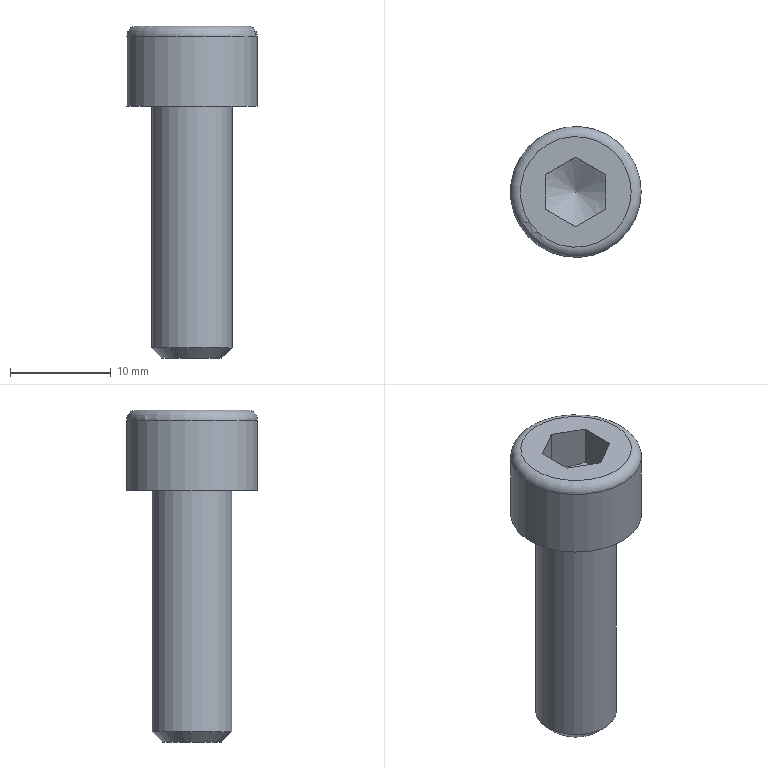Part | NX | features solid 2 | 1 solid | 14 faces | box 13 x 13 x 33 mm | volume 2150 mm3 | plane 9 | cylinder 2 | cone 2 | torus 1 | commonest cylinder face diameters 8 x1 13 x1
STEP:
#1=CARTESIAN_POINT('',(631.,-240.,30.));
#2=VERTEX_POINT('',#1);
#3=CARTESIAN_POINT('',(635.,-240.,30.));
#4=DIRECTION('',(0.,0.,-1.));
#5=DIRECTION('',(-1.,0.,0.));
#6=AXIS2_PLACEMENT_3D('',#3,#4,#5);
#7=CIRCLE('',#6,4.);
#8=EDGE_CURVE('',#2,#2,#7,.T.);
#9=ORIENTED_EDGE('',*,*,#8,.T.);
#10=EDGE_LOOP('',(#9));
#11=FACE_BOUND('',#10,.T.);
#12=CARTESIAN_POINT('',(631.,-240.,6.));
#13=VERTEX_POINT('',#12);
#14=CARTESIAN_POINT('',(635.,-240.,6.));
#15=DIRECTION('',(0.,0.,-1.));
#16=DIRECTION('',(-1.,0.,0.));
#17=AXIS2_PLACEMENT_3D('',#14,#15,#16);
#18=CIRCLE('',#17,4.);
#19=EDGE_CURVE('',#13,#13,#18,.F.);
#20=ORIENTED_EDGE('',*,*,#19,.T.);
#21=EDGE_LOOP('',(#20));
#22=FACE_BOUND('',#21,.T.);
#23=CARTESIAN_POINT('',(635.,-240.,30.));
#24=DIRECTION('',(0.,0.,-1.));
#25=DIRECTION('',(-1.,0.,0.));
#26=AXIS2_PLACEMENT_3D('',#23,#24,#25);
#27=CYLINDRICAL_SURFACE('',#26,4.);
#28=ADVANCED_FACE('',(#11,#22),#27,.T.);
#29=CARTESIAN_POINT('',(640.5,-240.,38.));
#30=VERTEX_POINT('',#29);
#31=CARTESIAN_POINT('',(635.,-240.,38.));
#32=DIRECTION('',(0.,0.,1.));
#33=DIRECTION('',(1.,0.,0.));
#34=AXIS2_PLACEMENT_3D('',#31,#32,#33);
#35=CIRCLE('',#34,5.5);
#36=EDGE_CURVE('',#30,#30,#35,.T.);
#37=ORIENTED_EDGE('',*,*,#36,.T.);
#38=EDGE_LOOP('',(#37));
#39=FACE_BOUND('',#38,.T.);
#40=CARTESIAN_POINT('',(638.,-241.732,38.));
#41=VERTEX_POINT('',#40);
#42=CARTESIAN_POINT('',(635.,-243.464,38.));
#43=VERTEX_POINT('',#42);
#44=CARTESIAN_POINT('',(638.,-241.732,38.));
#45=DIRECTION('',(-0.866,-0.5,0.));
#46=VECTOR('',#45,1000.);
#47=LINE('',#44,#46);
#48=EDGE_CURVE('',#41,#43,#47,.T.);
#49=ORIENTED_EDGE('',*,*,#48,.T.);
#50=CARTESIAN_POINT('',(632.,-241.732,38.));
#51=VERTEX_POINT('',#50);
#52=CARTESIAN_POINT('',(635.,-243.464,38.));
#53=DIRECTION('',(-0.866,0.5,0.));
#54=VECTOR('',#53,1000.);
#55=LINE('',#52,#54);
#56=EDGE_CURVE('',#43,#51,#55,.T.);
#57=ORIENTED_EDGE('',*,*,#56,.T.);
#58=CARTESIAN_POINT('',(632.,-238.268,38.));
#59=VERTEX_POINT('',#58);
#60=CARTESIAN_POINT('',(632.,-241.732,38.));
#61=DIRECTION('',(0.,1.,0.));
#62=VECTOR('',#61,1000.);
#63=LINE('',#60,#62);
#64=EDGE_CURVE('',#51,#59,#63,.T.);
#65=ORIENTED_EDGE('',*,*,#64,.T.);
#66=CARTESIAN_POINT('',(635.,-236.536,38.));
#67=VERTEX_POINT('',#66);
#68=CARTESIAN_POINT('',(632.,-238.268,38.));
#69=DIRECTION('',(0.866,0.5,0.));
#70=VECTOR('',#69,1000.);
#71=LINE('',#68,#70);
#72=EDGE_CURVE('',#59,#67,#71,.T.);
#73=ORIENTED_EDGE('',*,*,#72,.T.);
#74=CARTESIAN_POINT('',(638.,-238.268,38.));
#75=VERTEX_POINT('',#74);
#76=CARTESIAN_POINT('',(635.,-236.536,38.));
#77=DIRECTION('',(0.866,-0.5,0.));
#78=VECTOR('',#77,1000.);
#79=LINE('',#76,#78);
#80=EDGE_CURVE('',#67,#75,#79,.T.);
#81=ORIENTED_EDGE('',*,*,#80,.T.);
#82=CARTESIAN_POINT('',(638.,-238.268,38.));
#83=DIRECTION('',(0.,-1.,0.));
#84=VECTOR('',#83,1000.);
#85=LINE('',#82,#84);
#86=EDGE_CURVE('',#75,#41,#85,.T.);
#87=ORIENTED_EDGE('',*,*,#86,.T.);
#88=EDGE_LOOP('',(#49,#57,#65,#73,#81,#87));
#89=FACE_BOUND('',#88,.T.);
#90=CARTESIAN_POINT('',(635.,-240.,38.));
#91=DIRECTION('',(0.,0.,1.));
#92=DIRECTION('',(1.,0.,0.));
#93=AXIS2_PLACEMENT_3D('',#90,#91,#92);
#94=PLANE('',#93);
#95=ADVANCED_FACE('',(#39,#89),#94,.T.);
#96=ORIENTED_EDGE('',*,*,#8,.F.);
#97=EDGE_LOOP('',(#96));
#98=FACE_BOUND('',#97,.T.);
#99=CARTESIAN_POINT('',(641.5,-240.,30.));
#100=VERTEX_POINT('',#99);
#101=CARTESIAN_POINT('',(635.,-240.,30.));
#102=DIRECTION('',(0.,0.,1.));
#103=DIRECTION('',(1.,0.,0.));
#104=AXIS2_PLACEMENT_3D('',#101,#102,#103);
#105=CIRCLE('',#104,6.5);
#106=EDGE_CURVE('',#100,#100,#105,.T.);
#107=ORIENTED_EDGE('',*,*,#106,.F.);
#108=EDGE_LOOP('',(#107));
#109=FACE_BOUND('',#108,.T.);
#110=CARTESIAN_POINT('',(635.,-240.,30.));
#111=DIRECTION('',(0.,0.,-1.));
#112=DIRECTION('',(-1.,0.,0.));
#113=AXIS2_PLACEMENT_3D('',#110,#111,#112);
#114=PLANE('',#113);
#115=ADVANCED_FACE('',(#98,#109),#114,.T.);
#116=CARTESIAN_POINT('',(641.5,-240.,37.));
#117=VERTEX_POINT('',#116);
#118=CARTESIAN_POINT('',(635.,-240.,37.));
#119=DIRECTION('',(0.,0.,1.));
#120=DIRECTION('',(1.,0.,0.));
#121=AXIS2_PLACEMENT_3D('',#118,#119,#120);
#122=CIRCLE('',#121,6.5);
#123=EDGE_CURVE('',#117,#117,#122,.F.);
#124=ORIENTED_EDGE('',*,*,#123,.T.);
#125=EDGE_LOOP('',(#124));
#126=FACE_BOUND('',#125,.T.);
#127=ORIENTED_EDGE('',*,*,#106,.T.);
#128=EDGE_LOOP('',(#127));
#129=FACE_BOUND('',#128,.T.);
#130=CARTESIAN_POINT('',(635.,-240.,30.));
#131=DIRECTION('',(0.,0.,1.));
#132=DIRECTION('',(1.,0.,0.));
#133=AXIS2_PLACEMENT_3D('',#130,#131,#132);
#134=CYLINDRICAL_SURFACE('',#133,6.5);
#135=ADVANCED_FACE('',(#126,#129),#134,.T.);
#136=CARTESIAN_POINT('',(635.,-243.464,34.));
#137=VERTEX_POINT('',#136);
#138=CARTESIAN_POINT('',(635.,-243.464,38.));
#139=DIRECTION('',(0.,0.,-1.));
#140=VECTOR('',#139,1000.);
#141=LINE('',#138,#140);
#142=EDGE_CURVE('',#43,#137,#141,.T.);
#143=ORIENTED_EDGE('',*,*,#142,.F.);
#144=ORIENTED_EDGE('',*,*,#48,.F.);
#145=CARTESIAN_POINT('',(638.,-241.732,34.));
#146=VERTEX_POINT('',#145);
#147=CARTESIAN_POINT('',(638.,-241.732,38.));
#148=DIRECTION('',(0.,0.,-1.));
#149=VECTOR('',#148,1000.);
#150=LINE('',#147,#149);
#151=EDGE_CURVE('',#41,#146,#150,.T.);
#152=ORIENTED_EDGE('',*,*,#151,.T.);
#153=CARTESIAN_POINT('',(635.,-243.464,34.));
#154=CARTESIAN_POINT('',(635.98,-242.898,33.673));
#155=CARTESIAN_POINT('',(637.019,-242.298,33.673));
#156=CARTESIAN_POINT('',(638.,-241.732,34.));
#157=B_SPLINE_CURVE_WITH_KNOTS('',3,(#153,#154,#155,#156),.UNSPECIFIED.,.F.,.F.,(4,4),(0.000000238,0.003499),.UNSPECIFIED.);
#158=EDGE_CURVE('',#137,#146,#157,.T.);
#159=ORIENTED_EDGE('',*,*,#158,.F.);
#160=EDGE_LOOP('',(#143,#144,#152,#159));
#161=FACE_BOUND('',#160,.T.);
#162=CARTESIAN_POINT('',(636.5,-242.598,35.));
#163=DIRECTION('',(0.5,-0.866,0.));
#164=DIRECTION('',(0.866,0.5,0.));
#165=AXIS2_PLACEMENT_3D('',#162,#163,#164);
#166=PLANE('',#165);
#167=ADVANCED_FACE('',(#161),#166,.F.);
#168=ORIENTED_EDGE('',*,*,#151,.F.);
#169=ORIENTED_EDGE('',*,*,#86,.F.);
#170=CARTESIAN_POINT('',(638.,-238.268,34.));
#171=VERTEX_POINT('',#170);
#172=CARTESIAN_POINT('',(638.,-238.268,38.));
#173=DIRECTION('',(0.,0.,-1.));
#174=VECTOR('',#173,1000.);
#175=LINE('',#172,#174);
#176=EDGE_CURVE('',#75,#171,#175,.T.);
#177=ORIENTED_EDGE('',*,*,#176,.T.);
#178=CARTESIAN_POINT('',(638.,-241.732,34.));
#179=CARTESIAN_POINT('',(638.,-240.603,33.674));
#180=CARTESIAN_POINT('',(638.,-239.388,33.677));
#181=CARTESIAN_POINT('',(638.,-238.268,34.));
#182=B_SPLINE_CURVE_WITH_KNOTS('',3,(#178,#179,#180,#181),.UNSPECIFIED.,.F.,.F.,(4,4),(0.003209,0.006718),.UNSPECIFIED.);
#183=EDGE_CURVE('',#146,#171,#182,.T.);
#184=ORIENTED_EDGE('',*,*,#183,.F.);
#185=EDGE_LOOP('',(#168,#169,#177,#184));
#186=FACE_BOUND('',#185,.T.);
#187=CARTESIAN_POINT('',(638.,-240.,35.));
#188=DIRECTION('',(1.,0.,0.));
#189=DIRECTION('',(0.,0.,-1.));
#190=AXIS2_PLACEMENT_3D('',#187,#188,#189);
#191=PLANE('',#190);
#192=ADVANCED_FACE('',(#186),#191,.F.);
#193=ORIENTED_EDGE('',*,*,#176,.F.);
#194=ORIENTED_EDGE('',*,*,#80,.F.);
#195=CARTESIAN_POINT('',(635.,-236.536,34.));
#196=VERTEX_POINT('',#195);
#197=CARTESIAN_POINT('',(635.,-236.536,38.));
#198=DIRECTION('',(0.,0.,-1.));
#199=VECTOR('',#198,1000.);
#200=LINE('',#197,#199);
#201=EDGE_CURVE('',#67,#196,#200,.T.);
#202=ORIENTED_EDGE('',*,*,#201,.T.);
#203=CARTESIAN_POINT('',(638.,-238.268,34.));
#204=CARTESIAN_POINT('',(637.02,-237.702,33.673));
#205=CARTESIAN_POINT('',(635.981,-237.102,33.673));
#206=CARTESIAN_POINT('',(635.,-236.536,34.));
#207=B_SPLINE_CURVE_WITH_KNOTS('',3,(#203,#204,#205,#206),.UNSPECIFIED.,.F.,.F.,(4,4),(0.000000238,0.003499),.UNSPECIFIED.);
#208=EDGE_CURVE('',#171,#196,#207,.T.);
#209=ORIENTED_EDGE('',*,*,#208,.F.);
#210=EDGE_LOOP('',(#193,#194,#202,#209));
#211=FACE_BOUND('',#210,.T.);
#212=CARTESIAN_POINT('',(636.5,-237.402,35.));
#213=DIRECTION('',(0.5,0.866,0.));
#214=DIRECTION('',(-0.866,0.5,0.));
#215=AXIS2_PLACEMENT_3D('',#212,#213,#214);
#216=PLANE('',#215);
#217=ADVANCED_FACE('',(#211),#216,.F.);
#218=ORIENTED_EDGE('',*,*,#201,.F.);
#219=ORIENTED_EDGE('',*,*,#72,.F.);
#220=CARTESIAN_POINT('',(632.,-238.268,34.));
#221=VERTEX_POINT('',#220);
#222=CARTESIAN_POINT('',(632.,-238.268,38.));
#223=DIRECTION('',(0.,0.,-1.));
#224=VECTOR('',#223,1000.);
#225=LINE('',#222,#224);
#226=EDGE_CURVE('',#59,#221,#225,.T.);
#227=ORIENTED_EDGE('',*,*,#226,.T.);
#228=CARTESIAN_POINT('',(635.,-236.536,34.));
#229=CARTESIAN_POINT('',(634.02,-237.102,33.673));
#230=CARTESIAN_POINT('',(632.981,-237.702,33.673));
#231=CARTESIAN_POINT('',(632.,-238.268,34.));
#232=B_SPLINE_CURVE_WITH_KNOTS('',3,(#228,#229,#230,#231),.UNSPECIFIED.,.F.,.F.,(4,4),(0.000000238,0.003499),.UNSPECIFIED.);
#233=EDGE_CURVE('',#196,#221,#232,.T.);
#234=ORIENTED_EDGE('',*,*,#233,.F.);
#235=EDGE_LOOP('',(#218,#219,#227,#234));
#236=FACE_BOUND('',#235,.T.);
#237=CARTESIAN_POINT('',(633.5,-237.402,35.));
#238=DIRECTION('',(-0.5,0.866,0.));
#239=DIRECTION('',(-0.866,-0.5,0.));
#240=AXIS2_PLACEMENT_3D('',#237,#238,#239);
#241=PLANE('',#240);
#242=ADVANCED_FACE('',(#236),#241,.F.);
#243=ORIENTED_EDGE('',*,*,#226,.F.);
#244=ORIENTED_EDGE('',*,*,#64,.F.);
#245=CARTESIAN_POINT('',(632.,-241.732,34.));
#246=VERTEX_POINT('',#245);
#247=CARTESIAN_POINT('',(632.,-241.732,38.));
#248=DIRECTION('',(0.,0.,-1.));
#249=VECTOR('',#248,1000.);
#250=LINE('',#247,#249);
#251=EDGE_CURVE('',#51,#246,#250,.T.);
#252=ORIENTED_EDGE('',*,*,#251,.T.);
#253=CARTESIAN_POINT('',(632.,-241.732,34.));
#254=CARTESIAN_POINT('',(632.,-240.603,33.674));
#255=CARTESIAN_POINT('',(632.,-239.388,33.677));
#256=CARTESIAN_POINT('',(632.,-238.268,34.));
#257=B_SPLINE_CURVE_WITH_KNOTS('',3,(#253,#254,#255,#256),.UNSPECIFIED.,.F.,.F.,(4,4),(0.003209,0.006718),.UNSPECIFIED.);
#258=EDGE_CURVE('',#221,#246,#257,.F.);
#259=ORIENTED_EDGE('',*,*,#258,.F.);
#260=EDGE_LOOP('',(#243,#244,#252,#259));
#261=FACE_BOUND('',#260,.T.);
#262=CARTESIAN_POINT('',(632.,-240.,35.));
#263=DIRECTION('',(-1.,0.,0.));
#264=DIRECTION('',(0.,0.,1.));
#265=AXIS2_PLACEMENT_3D('',#262,#263,#264);
#266=PLANE('',#265);
#267=ADVANCED_FACE('',(#261),#266,.F.);
#268=ORIENTED_EDGE('',*,*,#251,.F.);
#269=ORIENTED_EDGE('',*,*,#56,.F.);
#270=ORIENTED_EDGE('',*,*,#142,.T.);
#271=CARTESIAN_POINT('',(632.,-241.732,34.));
#272=CARTESIAN_POINT('',(632.98,-242.298,33.673));
#273=CARTESIAN_POINT('',(634.019,-242.898,33.673));
#274=CARTESIAN_POINT('',(635.,-243.464,34.));
#275=B_SPLINE_CURVE_WITH_KNOTS('',3,(#271,#272,#273,#274),.UNSPECIFIED.,.F.,.F.,(4,4),(0.000000238,0.003499),.UNSPECIFIED.);
#276=EDGE_CURVE('',#246,#137,#275,.T.);
#277=ORIENTED_EDGE('',*,*,#276,.F.);
#278=EDGE_LOOP('',(#268,#269,#270,#277));
#279=FACE_BOUND('',#278,.T.);
#280=CARTESIAN_POINT('',(633.5,-242.598,35.));
#281=DIRECTION('',(-0.5,-0.866,0.));
#282=DIRECTION('',(0.866,-0.5,0.));
#283=AXIS2_PLACEMENT_3D('',#280,#281,#282);
#284=PLANE('',#283);
#285=ADVANCED_FACE('',(#279),#284,.F.);
#286=ORIENTED_EDGE('',*,*,#158,.T.);
#287=ORIENTED_EDGE('',*,*,#183,.T.);
#288=ORIENTED_EDGE('',*,*,#208,.T.);
#289=ORIENTED_EDGE('',*,*,#233,.T.);
#290=ORIENTED_EDGE('',*,*,#258,.T.);
#291=ORIENTED_EDGE('',*,*,#276,.T.);
#292=EDGE_LOOP('',(#286,#287,#288,#289,#290,#291));
#293=FACE_BOUND('',#292,.T.);
#294=CARTESIAN_POINT('',(635.,-240.,32.));
#295=VERTEX_POINT('',#294);
#296=VERTEX_LOOP('',#295);
#297=FACE_BOUND('',#296,.T.);
#298=CARTESIAN_POINT('',(635.,-240.,32.));
#299=DIRECTION('',(0.,0.,1.));
#300=DIRECTION('',(1.,0.,0.));
#301=AXIS2_PLACEMENT_3D('',#298,#299,#300);
#302=CONICAL_SURFACE('',#301,0.,1.047);
#303=ADVANCED_FACE('',(#293,#297),#302,.F.);
#304=ORIENTED_EDGE('',*,*,#36,.F.);
#305=EDGE_LOOP('',(#304));
#306=FACE_BOUND('',#305,.T.);
#307=ORIENTED_EDGE('',*,*,#123,.F.);
#308=EDGE_LOOP('',(#307));
#309=FACE_BOUND('',#308,.T.);
#310=CARTESIAN_POINT('',(635.,-240.,37.));
#311=DIRECTION('',(0.,0.,1.));
#312=DIRECTION('',(1.,0.,0.));
#313=AXIS2_PLACEMENT_3D('',#310,#311,#312);
#314=TOROIDAL_SURFACE('',#313,5.5,1.);
#315=ADVANCED_FACE('',(#306,#309),#314,.T.);
#316=CARTESIAN_POINT('',(632.,-240.,5.));
#317=VERTEX_POINT('',#316);
#318=CARTESIAN_POINT('',(635.,-240.,5.));
#319=DIRECTION('',(0.,0.,-1.));
#320=DIRECTION('',(-1.,0.,0.));
#321=AXIS2_PLACEMENT_3D('',#318,#319,#320);
#322=CIRCLE('',#321,3.);
#323=EDGE_CURVE('',#317,#317,#322,.T.);
#324=ORIENTED_EDGE('',*,*,#323,.T.);
#325=EDGE_LOOP('',(#324));
#326=FACE_BOUND('',#325,.T.);
#327=CARTESIAN_POINT('',(635.,-240.,5.));
#328=DIRECTION('',(0.,0.,-1.));
#329=DIRECTION('',(-1.,0.,0.));
#330=AXIS2_PLACEMENT_3D('',#327,#328,#329);
#331=PLANE('',#330);
#332=ADVANCED_FACE('',(#326),#331,.T.);
#333=ORIENTED_EDGE('',*,*,#323,.F.);
#334=EDGE_LOOP('',(#333));
#335=FACE_BOUND('',#334,.T.);
#336=ORIENTED_EDGE('',*,*,#19,.F.);
#337=EDGE_LOOP('',(#336));
#338=FACE_BOUND('',#337,.T.);
#339=CARTESIAN_POINT('',(635.,-240.,6.));
#340=DIRECTION('',(0.,0.,1.));
#341=DIRECTION('',(1.,0.,0.));
#342=AXIS2_PLACEMENT_3D('',#339,#340,#341);
#343=CONICAL_SURFACE('',#342,4.,0.7854);
#344=ADVANCED_FACE('',(#335,#338),#343,.T.);
#345=CLOSED_SHELL('',(#28,#95,#115,#135,#167,#192,#217,#242,#267,#285,#303,#315,#332,#344));
#346=MANIFOLD_SOLID_BREP('',#345);
#347=(LENGTH_UNIT()NAMED_UNIT(*)SI_UNIT(.MILLI.,.METRE.));
#348=UNCERTAINTY_MEASURE_WITH_UNIT(LENGTH_MEASURE(0.0508),#347,'','');
#349=(NAMED_UNIT(*)PLANE_ANGLE_UNIT()SI_UNIT($,.RADIAN.));
#350=(NAMED_UNIT(*)SI_UNIT($,.STERADIAN.)SOLID_ANGLE_UNIT());
#351=(GEOMETRIC_REPRESENTATION_CONTEXT(3)GLOBAL_UNCERTAINTY_ASSIGNED_CONTEXT((#348))GLOBAL_UNIT_ASSIGNED_CONTEXT((#347,#349,#350))REPRESENTATION_CONTEXT('',''));
#352=ADVANCED_BREP_SHAPE_REPRESENTATION('',(#346),#351);